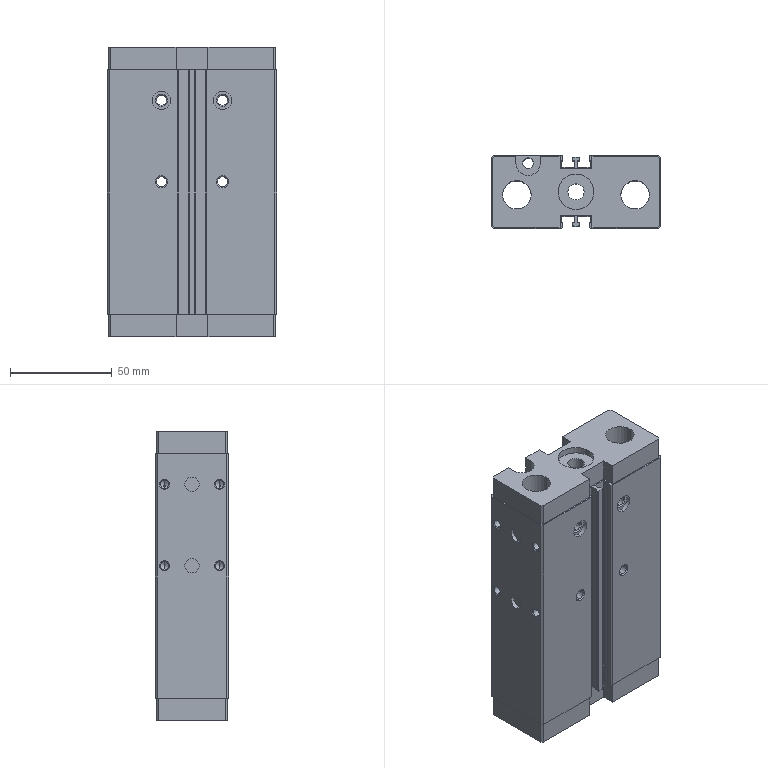Part | SolidWorks | features RefAxis 33, RevCut 25, 3DProfileFeature 11, ICE 4, Extrusion 1 | 1 solid | 239 faces | box 83 x 36 x 142 mm | volume 314811 mm3 | plane 105 | cylinder 98 | cone 36 | commonest cylinder face diameters 4.134 x20 0.4 x16 0.8 x14 9 x12 4.917 x8 5.3 x8